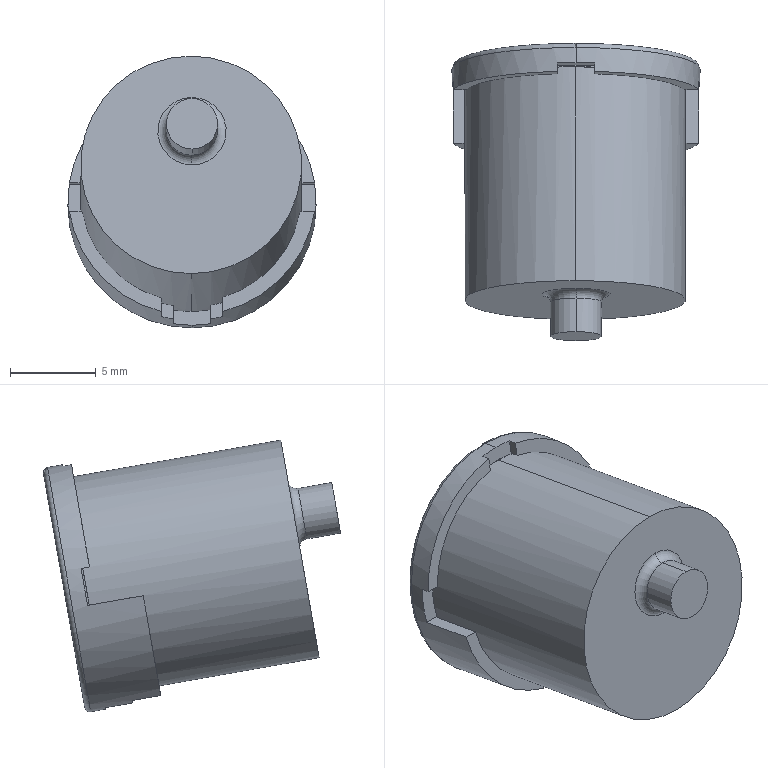Part | STEP file | _X2_751F4E45_X0_MS731-1_X2_8F_1 | 1 solid | 54 faces | box 14.5 x 17.374 x 15.879 mm | volume 1874 mm3 | plane 42 | cylinder 8 | torus 4 | commonest cylinder face diameters 3 x2 12.8 x2 12.906 x2 14.5 x2